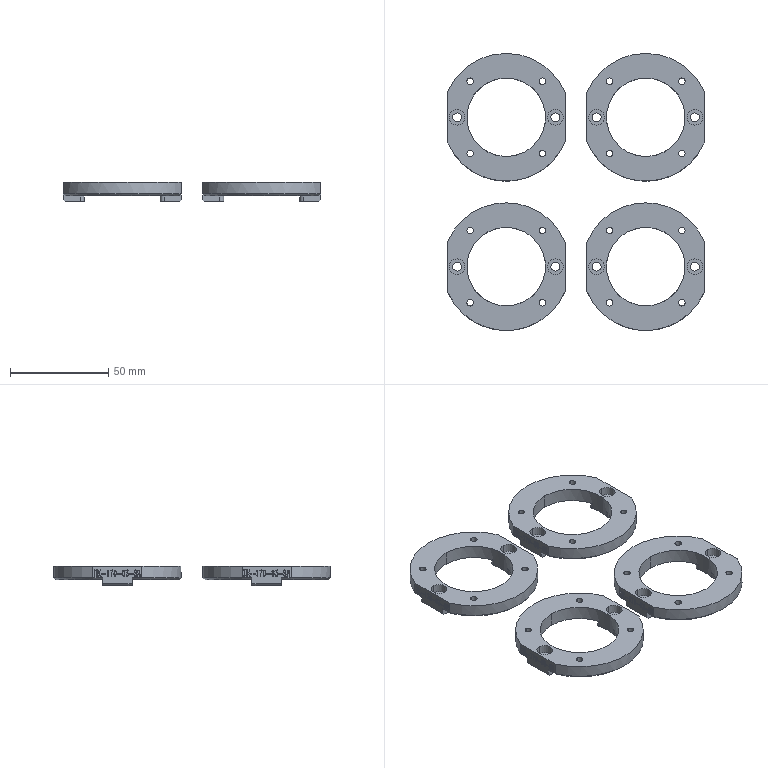NC program | NX | posted with a generic post | part box 131 x 141 x 10 mm
Lines 1 to 797 of 14293:
N10 G17 G21 G94 G90
(ZLEVEL_PROFILE_COPY_1_COPY , TOOL : D10)
N12 T15 M6
N14 G54
N16 G17 G0 G90 X-41.889 Y-75.045 S9500 M3
N18 G43 Z30. H15
N20 Z1.5
N22 G94 G1 X-42.763 Y-74.922 Z1.454 F1000.
N24 X-46.803 Y-73.892 Z1.235
N26 X-50.704 Y-72.422 Z1.017
N28 X-54.419 Y-70.528 Z0.798
N30 X-57.902 Y-68.235 Z0.58
N32 X-61.109 Y-65.572 Z0.361
N34 X-64.002 Y-62.569 Z0.143
N36 X-66.545 Y-59.265 Z-0.076
N38 X-68.143 Y-56.72 Z-0.233
N40 X-69.63 Y-53.848 Z-0.403
N42 X-70.208 Y-52.462 Z-0.482
N44 X-70.421 Y-51.95 Z-0.511
N46 X-70.6 Y-51.054 Z-0.558
N48 Y-50.5 Z-0.588
N50 Y-25.5 F3000.
N52 G2 X-70.208 Y-23.538 R5.1
N54 X-0.792 Y-23.538 R37.6
N56 X-0.4 Y-25.5 R5.1
N58 G1 Y-50.5
N60 G2 X-0.792 Y-52.462 R5.1
N62 X-70.208 Y-52.462 R37.6
N64 X-70.6 Y-50.5 R5.1
N66 G1 Y-25.5 Z-0.65
N68 X-70.575 Y-24.997 Z-0.651
N70 X-70.501 Y-24.5 Z-0.653
N72 X-70.378 Y-24.012 Z-0.654
N74 X-70.208 Y-23.538 Z-0.655
N76 X-69.614 Y-22.19 Z-0.659
N78 X-68.969 Y-20.865 Z-0.662
N80 X-68.272 Y-19.567 Z-0.666
N82 X-67.524 Y-18.297 Z-0.67
N84 X-66.727 Y-17.057 Z-0.673
N86 X-65.883 Y-15.85 Z-0.677
N88 X-64.992 Y-14.676 Z-0.681
N90 X-64.055 Y-13.538 Z-0.685
N92 X-63.075 Y-12.438 Z-0.688
N94 X-62.052 Y-11.377 Z-0.692
N96 X-60.988 Y-10.358 Z-0.696
N98 X-59.886 Y-9.38 Z-0.699
N100 X-58.745 Y-8.447 Z-0.703
N102 X-57.57 Y-7.558 Z-0.707
N104 X-56.36 Y-6.717 Z-0.71
N106 X-55.118 Y-5.924 Z-0.714
N108 X-53.846 Y-5.18 Z-0.718
N110 X-52.546 Y-4.486 Z-0.721
N112 X-51.22 Y-3.844 Z-0.725
N114 X-49.869 Y-3.254 Z-0.729
N116 X-48.497 Y-2.718 Z-0.732
N118 X-47.104 Y-2.235 Z-0.736
N120 X-45.694 Y-1.808 Z-0.74
N122 X-44.268 Y-1.437 Z-0.744
N124 X-42.829 Y-1.121 Z-0.747
N126 X-41.378 Y-0.862 Z-0.751
N128 X-39.918 Y-0.66 Z-0.755
N130 X-38.452 Y-0.516 Z-0.758
N132 X-36.981 Y-0.429 Z-0.762
N134 X-35.508 Y-0.4 Z-0.766
N136 X-34.034 Y-0.429 Z-0.769
N138 X-32.562 Y-0.515 Z-0.773
N140 X-31.095 Y-0.659 Z-0.777
N142 X-29.635 Y-0.86 Z-0.78
N144 X-28.184 Y-1.119 Z-0.784
N146 X-26.744 Y-1.434 Z-0.788
N148 X-25.317 Y-1.805 Z-0.791
N150 X-23.906 Y-2.232 Z-0.795
N152 X-22.513 Y-2.714 Z-0.799
N154 X-21.14 Y-3.25 Z-0.802
N156 X-19.789 Y-3.84 Z-0.806
N158 X-18.462 Y-4.482 Z-0.81
N160 X-17.161 Y-5.175 Z-0.814
N162 X-15.889 Y-5.919 Z-0.817
N164 X-14.646 Y-6.713 Z-0.821
N166 X-13.436 Y-7.554 Z-0.825
N168 X-12.26 Y-8.442 Z-0.828
N170 X-11.119 Y-9.376 Z-0.832
N172 X-10.016 Y-10.354 Z-0.836
N174 X-8.952 Y-11.374 Z-0.839
N176 X-7.928 Y-12.435 Z-0.843
N178 X-6.948 Y-13.535 Z-0.847
N180 X-6.011 Y-14.673 Z-0.85
N182 X-5.119 Y-15.847 Z-0.854
N184 X-4.274 Y-17.055 Z-0.858
N186 X-3.477 Y-18.295 Z-0.861
N188 X-2.729 Y-19.565 Z-0.865
N190 X-2.032 Y-20.864 Z-0.869
N192 X-1.386 Y-22.189 Z-0.873
N194 X-0.792 Y-23.538 Z-0.876
N196 X-0.622 Y-24.012 Z-0.877
N198 X-0.499 Y-24.5 Z-0.879
N200 X-0.425 Y-24.997 Z-0.88
N202 X-0.4 Y-25.5 Z-0.881
N204 Y-50.5 Z-0.944
N206 X-0.425 Y-51.003 Z-0.945
N208 X-0.499 Y-51.5 Z-0.946
N210 X-0.622 Y-51.988 Z-0.948
N212 X-0.792 Y-52.462 Z-0.949
N214 X-1.383 Y-53.805 Z-0.952
N216 X-2.026 Y-55.125 Z-0.956
N218 X-2.72 Y-56.418 Z-0.96
N220 X-3.464 Y-57.683 Z-0.963
N222 X-4.256 Y-58.919 Z-0.967
N224 X-5.097 Y-60.122 Z-0.971
N226 X-5.983 Y-61.292 Z-0.975
N228 X-6.915 Y-62.426 Z-0.978
N230 X-7.89 Y-63.523 Z-0.982
N232 X-8.907 Y-64.581 Z-0.986
N234 X-9.965 Y-65.599 Z-0.989
N236 X-11.061 Y-66.575 Z-0.993
N238 X-12.195 Y-67.507 Z-0.997
N240 X-13.364 Y-68.394 Z-1.
N242 X-14.568 Y-69.234 Z-1.004
N244 X-15.803 Y-70.028 Z-1.008
N246 X-17.068 Y-70.772 Z-1.011
N248 X-18.361 Y-71.466 Z-1.015
N250 X-19.68 Y-72.11 Z-1.019
N252 X-21.023 Y-72.701 Z-1.022
N254 X-22.389 Y-73.24 Z-1.026
N256 X-23.774 Y-73.725 Z-1.03
N258 X-25.177 Y-74.155 Z-1.033
N260 X-26.596 Y-74.531 Z-1.037
N262 X-28.029 Y-74.85 Z-1.041
N264 X-29.473 Y-75.114 Z-1.044
N266 X-30.926 Y-75.321 Z-1.048
N268 X-32.386 Y-75.471 Z-1.052
N270 X-33.851 Y-75.564 Z-1.055
N272 X-35.318 Y-75.6 Z-1.059
N274 X-36.786 Y-75.578 Z-1.063
N276 X-38.251 Y-75.499 Z-1.066
N278 X-39.713 Y-75.363 Z-1.07
N280 X-41.168 Y-75.17 Z-1.074
N282 X-42.614 Y-74.921 Z-1.077
N284 X-44.05 Y-74.615 Z-1.081
N286 X-45.472 Y-74.254 Z-1.085
N288 X-46.879 Y-73.837 Z-1.088
N290 X-48.269 Y-73.365 Z-1.092
N292 X-49.64 Y-72.84 Z-1.096
N294 X-50.989 Y-72.262 Z-1.099
N296 X-52.314 Y-71.631 Z-1.103
N298 X-53.614 Y-70.949 Z-1.107
N300 X-54.886 Y-70.217 Z-1.11
N302 X-56.129 Y-69.436 Z-1.114
N304 X-57.34 Y-68.607 Z-1.118
N306 X-58.518 Y-67.731 Z-1.121
N308 X-59.661 Y-66.81 Z-1.125
N310 X-60.767 Y-65.845 Z-1.129
N312 X-61.834 Y-64.838 Z-1.132
N314 X-62.862 Y-63.789 Z-1.136
N316 X-63.847 Y-62.702 Z-1.14
N318 X-64.79 Y-61.577 Z-1.143
N320 X-65.688 Y-60.416 Z-1.147
N322 X-66.54 Y-59.22 Z-1.151
N324 X-67.344 Y-57.993 Z-1.154
N326 X-67.885 Y-57.105 Z-1.157
N328 X-68.4 Y-56.203 Z-1.16
N330 X-68.891 Y-55.287 Z-1.162
N332 X-69.356 Y-54.357 Z-1.165
N334 X-69.795 Y-53.415 Z-1.167
N336 X-70.208 Y-52.462 Z-1.17
N338 X-70.378 Y-51.988 Z-1.171
N340 X-70.501 Y-51.5 Z-1.172
N342 X-70.575 Y-51.003 Z-1.174
N344 X-70.6 Y-50.5 Z-1.175
N346 Y-25.5 Z-1.238
N348 X-70.575 Y-24.997 Z-1.239
N350 X-70.501 Y-24.5 Z-1.24
N352 X-70.378 Y-24.012 Z-1.241
N354 X-70.208 Y-23.538 Z-1.243
N356 X-69.614 Y-22.19 Z-1.246
N358 X-68.969 Y-20.865 Z-1.25
N360 X-68.272 Y-19.567 Z-1.254
N362 X-67.524 Y-18.297 Z-1.257
N364 X-66.727 Y-17.057 Z-1.261
N366 X-65.883 Y-15.85 Z-1.265
N368 X-64.992 Y-14.676 Z-1.268
N370 X-64.055 Y-13.538 Z-1.272
N372 X-63.075 Y-12.438 Z-1.276
N374 X-62.052 Y-11.377 Z-1.279
N376 X-60.988 Y-10.358 Z-1.283
N378 X-59.886 Y-9.38 Z-1.287
N380 X-58.745 Y-8.447 Z-1.29
N382 X-57.57 Y-7.558 Z-1.294
N384 X-56.36 Y-6.717 Z-1.298
N386 X-55.118 Y-5.924 Z-1.302
N388 X-53.846 Y-5.18 Z-1.305
N390 X-52.546 Y-4.486 Z-1.309
N392 X-51.22 Y-3.844 Z-1.313
N394 X-49.869 Y-3.254 Z-1.316
N396 X-48.497 Y-2.718 Z-1.32
N398 X-47.104 Y-2.235 Z-1.324
N400 X-45.694 Y-1.808 Z-1.327
N402 X-44.268 Y-1.437 Z-1.331
N404 X-42.829 Y-1.121 Z-1.335
N406 X-41.378 Y-0.862 Z-1.338
N408 X-39.918 Y-0.66 Z-1.342
N410 X-38.452 Y-0.516 Z-1.346
N412 X-36.981 Y-0.429 Z-1.349
N414 X-35.508 Y-0.4 Z-1.353
N416 X-34.034 Y-0.429 Z-1.357
N418 X-32.562 Y-0.515 Z-1.36
N420 X-31.095 Y-0.659 Z-1.364
N422 X-29.635 Y-0.86 Z-1.368
N424 X-28.184 Y-1.119 Z-1.372
N426 X-26.744 Y-1.434 Z-1.375
N428 X-25.317 Y-1.805 Z-1.379
N430 X-23.906 Y-2.232 Z-1.383
N432 X-22.513 Y-2.714 Z-1.386
N434 X-21.14 Y-3.25 Z-1.39
N436 X-19.789 Y-3.84 Z-1.394
N438 X-18.462 Y-4.482 Z-1.397
N440 X-17.161 Y-5.175 Z-1.401
N442 X-15.889 Y-5.919 Z-1.405
N444 X-14.646 Y-6.713 Z-1.408
N446 X-13.436 Y-7.554 Z-1.412
N448 X-12.26 Y-8.442 Z-1.416
N450 X-11.119 Y-9.376 Z-1.419
N452 X-10.016 Y-10.354 Z-1.423
N454 X-8.952 Y-11.374 Z-1.427
N456 X-7.928 Y-12.435 Z-1.431
N458 X-6.948 Y-13.535 Z-1.434
N460 X-6.011 Y-14.673 Z-1.438
N462 X-5.119 Y-15.847 Z-1.442
N464 X-4.274 Y-17.055 Z-1.445
N466 X-3.477 Y-18.295 Z-1.449
N468 X-2.729 Y-19.565 Z-1.453
N470 X-2.032 Y-20.864 Z-1.456
N472 X-1.386 Y-22.189 Z-1.46
N474 X-0.792 Y-23.538 Z-1.464
N476 X-0.622 Y-24.012 Z-1.465
N478 X-0.499 Y-24.5 Z-1.466
N480 X-0.425 Y-24.997 Z-1.467
N482 X-0.4 Y-25.5 Z-1.469
N484 Y-50.5 Z-1.531
N486 X-0.425 Y-51.003 Z-1.533
N488 X-0.499 Y-51.5 Z-1.534
N490 X-0.622 Y-51.988 Z-1.535
N492 X-0.792 Y-52.462 Z-1.536
N494 X-1.383 Y-53.805 Z-1.54
N496 X-2.026 Y-55.125 Z-1.544
N498 X-2.72 Y-56.418 Z-1.547
N500 X-3.464 Y-57.683 Z-1.551
N502 X-4.256 Y-58.919 Z-1.555
N504 X-5.097 Y-60.122 Z-1.558
N506 X-5.983 Y-61.292 Z-1.562
N508 X-6.915 Y-62.426 Z-1.566
N510 X-7.89 Y-63.523 Z-1.569
N512 X-8.907 Y-64.581 Z-1.573
N514 X-9.965 Y-65.599 Z-1.577
N516 X-11.061 Y-66.575 Z-1.58
N518 X-12.195 Y-67.507 Z-1.584
N520 X-13.364 Y-68.394 Z-1.588
N522 X-14.568 Y-69.234 Z-1.591
N524 X-15.803 Y-70.028 Z-1.595
N526 X-17.068 Y-70.772 Z-1.599
N528 X-18.361 Y-71.466 Z-1.602
N530 X-19.68 Y-72.11 Z-1.606
N532 X-21.023 Y-72.701 Z-1.61
N534 X-22.389 Y-73.24 Z-1.613
N536 X-23.774 Y-73.725 Z-1.617
N538 X-25.177 Y-74.155 Z-1.621
N540 X-26.596 Y-74.531 Z-1.624
N542 X-28.029 Y-74.85 Z-1.628
N544 X-29.473 Y-75.114 Z-1.632
N546 X-30.926 Y-75.321 Z-1.635
N548 X-32.386 Y-75.471 Z-1.639
N550 X-33.851 Y-75.564 Z-1.643
N552 X-35.318 Y-75.6 Z-1.646
N554 X-36.786 Y-75.578 Z-1.65
N556 X-38.251 Y-75.499 Z-1.654
N558 X-39.713 Y-75.363 Z-1.657
N560 X-41.168 Y-75.17 Z-1.661
N562 X-42.614 Y-74.921 Z-1.665
N564 X-44.05 Y-74.615 Z-1.668
N566 X-45.472 Y-74.254 Z-1.672
N568 X-46.879 Y-73.837 Z-1.676
N570 X-48.269 Y-73.365 Z-1.679
N572 X-49.64 Y-72.84 Z-1.683
N574 X-50.989 Y-72.262 Z-1.687
N576 X-52.314 Y-71.631 Z-1.69
N578 X-53.614 Y-70.949 Z-1.694
N580 X-54.886 Y-70.217 Z-1.698
N582 X-56.129 Y-69.436 Z-1.701
N584 X-57.34 Y-68.607 Z-1.705
N586 X-58.518 Y-67.731 Z-1.709
N588 X-59.661 Y-66.81 Z-1.713
N590 X-60.767 Y-65.845 Z-1.716
N592 X-61.834 Y-64.838 Z-1.72
N594 X-62.862 Y-63.789 Z-1.724
N596 X-63.847 Y-62.702 Z-1.727
N598 X-64.79 Y-61.577 Z-1.731
N600 X-65.688 Y-60.416 Z-1.735
N602 X-66.54 Y-59.22 Z-1.738
N604 X-67.344 Y-57.993 Z-1.742
N606 X-67.885 Y-57.105 Z-1.744
N608 X-68.4 Y-56.203 Z-1.747
N610 X-68.891 Y-55.287 Z-1.75
N612 X-69.356 Y-54.357 Z-1.752
N614 X-69.795 Y-53.415 Z-1.755
N616 X-70.208 Y-52.462 Z-1.757
N618 X-70.378 Y-51.988 Z-1.759
N620 X-70.501 Y-51.5 Z-1.76
N622 X-70.575 Y-51.003 Z-1.761
N624 X-70.6 Y-50.5 Z-1.763
N626 Y-25.5 Z-1.825
N628 X-70.575 Y-24.997 Z-1.826
N630 X-70.501 Y-24.5 Z-1.828
N632 X-70.378 Y-24.012 Z-1.829
N634 X-70.208 Y-23.538 Z-1.83
N636 X-69.614 Y-22.19 Z-1.834
N638 X-68.969 Y-20.865 Z-1.837
N640 X-68.272 Y-19.567 Z-1.841
N642 X-67.524 Y-18.297 Z-1.845
N644 X-66.727 Y-17.057 Z-1.848
N646 X-65.883 Y-15.85 Z-1.852
N648 X-64.992 Y-14.676 Z-1.856
N650 X-64.055 Y-13.538 Z-1.86
N652 X-63.075 Y-12.438 Z-1.863
N654 X-62.052 Y-11.377 Z-1.867
N656 X-60.988 Y-10.358 Z-1.871
N658 X-59.886 Y-9.38 Z-1.874
N660 X-58.745 Y-8.447 Z-1.878
N662 X-57.57 Y-7.558 Z-1.882
N664 X-56.36 Y-6.717 Z-1.885
N666 X-55.118 Y-5.924 Z-1.889
N668 X-53.846 Y-5.18 Z-1.893
N670 X-52.546 Y-4.486 Z-1.896
N672 X-51.22 Y-3.844 Z-1.9
N674 X-49.869 Y-3.254 Z-1.904
N676 X-48.497 Y-2.718 Z-1.907
N678 X-47.104 Y-2.235 Z-1.911
N680 X-45.694 Y-1.808 Z-1.915
N682 X-44.268 Y-1.437 Z-1.919
N684 X-42.829 Y-1.121 Z-1.922
N686 X-41.378 Y-0.862 Z-1.926
N688 X-39.918 Y-0.66 Z-1.93
N690 X-38.452 Y-0.516 Z-1.933
N692 X-36.981 Y-0.429 Z-1.937
N694 X-35.508 Y-0.4 Z-1.941
N696 X-34.034 Y-0.429 Z-1.944
N698 X-32.562 Y-0.515 Z-1.948
N700 X-31.095 Y-0.659 Z-1.952
N702 X-29.635 Y-0.86 Z-1.955
N704 X-28.184 Y-1.119 Z-1.959
N706 X-26.744 Y-1.434 Z-1.963
N708 X-25.317 Y-1.805 Z-1.966
N710 X-23.906 Y-2.232 Z-1.97
N712 X-22.513 Y-2.714 Z-1.974
N714 X-21.14 Y-3.25 Z-1.977
N716 X-19.789 Y-3.84 Z-1.981
N718 X-18.462 Y-4.482 Z-1.985
N720 X-17.161 Y-5.175 Z-1.989
N722 X-15.889 Y-5.919 Z-1.992
N724 X-14.646 Y-6.713 Z-1.996
N726 X-13.436 Y-7.554 Z-2.
N728 X-12.26 Y-8.442 Z-2.003
N730 X-11.119 Y-9.376 Z-2.007
N732 X-10.016 Y-10.354 Z-2.011
N734 X-8.952 Y-11.374 Z-2.014
N736 X-7.928 Y-12.435 Z-2.018
N738 X-6.948 Y-13.535 Z-2.022
N740 X-6.011 Y-14.673 Z-2.025
N742 X-5.119 Y-15.847 Z-2.029
N744 X-4.274 Y-17.055 Z-2.033
N746 X-3.477 Y-18.295 Z-2.036
N748 X-2.729 Y-19.565 Z-2.04
N750 X-2.032 Y-20.864 Z-2.044
N752 X-1.386 Y-22.189 Z-2.048
N754 X-0.792 Y-23.538 Z-2.051
N756 X-0.622 Y-24.012 Z-2.052
N758 X-0.499 Y-24.5 Z-2.054
N760 X-0.425 Y-24.997 Z-2.055
N762 X-0.4 Y-25.5 Z-2.056
N764 Y-50.5 Z-2.119
N766 X-0.425 Y-51.003 Z-2.12
N768 X-0.499 Y-51.5 Z-2.121
N770 X-0.622 Y-51.988 Z-2.123
N772 X-0.792 Y-52.462 Z-2.124
N774 X-1.383 Y-53.805 Z-2.127
N776 X-2.026 Y-55.125 Z-2.131
N778 X-2.72 Y-56.418 Z-2.135
N780 X-3.464 Y-57.683 Z-2.138
N782 X-4.256 Y-58.919 Z-2.142
N784 X-5.097 Y-60.122 Z-2.146
N786 X-5.983 Y-61.292 Z-2.15
N788 X-6.915 Y-62.426 Z-2.153
N790 X-7.89 Y-63.523 Z-2.157
N792 X-8.907 Y-64.581 Z-2.161
N794 X-9.965 Y-65.599 Z-2.164
N796 X-11.061 Y-66.575 Z-2.168
N798 X-12.195 Y-67.507 Z-2.172
N800 X-13.364 Y-68.394 Z-2.175
N802 X-14.568 Y-69.234 Z-2.179
N804 X-15.803 Y-70.028 Z-2.183
N806 X-17.068 Y-70.772 Z-2.186
N808 X-18.361 Y-71.466 Z-2.19
N810 X-19.68 Y-72.11 Z-2.194
N812 X-21.023 Y-72.701 Z-2.197
N814 X-22.389 Y-73.24 Z-2.201
N816 X-23.774 Y-73.725 Z-2.205
N818 X-25.177 Y-74.155 Z-2.208
N820 X-26.596 Y-74.531 Z-2.212
N822 X-28.029 Y-74.85 Z-2.216
N824 X-29.473 Y-75.114 Z-2.219
N826 X-30.926 Y-75.321 Z-2.223
N828 X-32.386 Y-75.471 Z-2.227
N830 X-33.851 Y-75.564 Z-2.23
N832 X-35.318 Y-75.6 Z-2.234
N834 X-36.786 Y-75.578 Z-2.238
N836 X-38.251 Y-75.499 Z-2.241
N838 X-39.713 Y-75.363 Z-2.245
N840 X-41.168 Y-75.17 Z-2.249
N842 X-42.614 Y-74.921 Z-2.252
N844 X-44.05 Y-74.615 Z-2.256
N846 X-45.472 Y-74.254 Z-2.26
N848 X-46.879 Y-73.837 Z-2.263
N850 X-48.269 Y-73.365 Z-2.267
N852 X-49.64 Y-72.84 Z-2.271
N854 X-50.989 Y-72.262 Z-2.274
N856 X-52.314 Y-71.631 Z-2.278
N858 X-53.614 Y-70.949 Z-2.282
N860 X-54.886 Y-70.217 Z-2.285
N862 X-56.129 Y-69.436 Z-2.289
N864 X-57.34 Y-68.607 Z-2.293
N866 X-58.518 Y-67.731 Z-2.296
N868 X-59.661 Y-66.81 Z-2.3
N870 X-60.767 Y-65.845 Z-2.304
N872 X-61.834 Y-64.838 Z-2.307
N874 X-62.862 Y-63.789 Z-2.311
N876 X-63.847 Y-62.702 Z-2.315
N878 X-64.79 Y-61.577 Z-2.318
N880 X-65.688 Y-60.416 Z-2.322
N882 X-66.54 Y-59.22 Z-2.326
N884 X-67.344 Y-57.993 Z-2.329
N886 X-67.885 Y-57.105 Z-2.332
N888 X-68.4 Y-56.203 Z-2.335
N890 X-68.891 Y-55.287 Z-2.337
N892 X-69.356 Y-54.357 Z-2.34
N894 X-69.795 Y-53.415 Z-2.342
N896 X-70.208 Y-52.462 Z-2.345
N898 X-70.378 Y-51.988 Z-2.346
N900 X-70.501 Y-51.5 Z-2.347
N902 X-70.575 Y-51.003 Z-2.349
N904 X-70.6 Y-50.5 Z-2.35
N906 Y-25.5 Z-2.413
N908 X-70.575 Y-24.997 Z-2.414
N910 X-70.501 Y-24.5 Z-2.415
N912 X-70.378 Y-24.012 Z-2.416
N914 X-70.208 Y-23.538 Z-2.418
N916 X-69.614 Y-22.19 Z-2.421
N918 X-68.969 Y-20.865 Z-2.425
N920 X-68.272 Y-19.567 Z-2.429
N922 X-67.524 Y-18.297 Z-2.432
N924 X-66.727 Y-17.057 Z-2.436
N926 X-65.883 Y-15.85 Z-2.44
N928 X-64.992 Y-14.676 Z-2.443
N930 X-64.055 Y-13.538 Z-2.447
N932 X-63.075 Y-12.438 Z-2.451
N934 X-62.052 Y-11.377 Z-2.454
N936 X-60.988 Y-10.358 Z-2.458
N938 X-59.886 Y-9.38 Z-2.462
N940 X-58.745 Y-8.447 Z-2.465
N942 X-57.57 Y-7.558 Z-2.469
N944 X-56.36 Y-6.717 Z-2.473
N946 X-55.118 Y-5.924 Z-2.477
N948 X-53.846 Y-5.18 Z-2.48
N950 X-52.546 Y-4.486 Z-2.484
N952 X-51.22 Y-3.844 Z-2.488
N954 X-49.869 Y-3.254 Z-2.491
N956 X-48.497 Y-2.718 Z-2.495
N958 X-47.104 Y-2.235 Z-2.499
N960 X-45.694 Y-1.808 Z-2.502
N962 X-44.268 Y-1.437 Z-2.506
N964 X-42.829 Y-1.121 Z-2.51
N966 X-41.378 Y-0.862 Z-2.513
N968 X-39.918 Y-0.66 Z-2.517
N970 X-38.452 Y-0.516 Z-2.521
N972 X-36.981 Y-0.429 Z-2.524
N974 X-35.508 Y-0.4 Z-2.528
N976 X-34.034 Y-0.429 Z-2.532
N978 X-32.562 Y-0.515 Z-2.535
N980 X-31.095 Y-0.659 Z-2.539
N982 X-29.635 Y-0.86 Z-2.543
N984 X-28.184 Y-1.119 Z-2.547
N986 X-26.744 Y-1.434 Z-2.55
N988 X-25.317 Y-1.805 Z-2.554
N990 X-23.906 Y-2.232 Z-2.558
N992 X-22.513 Y-2.714 Z-2.561
N994 X-21.14 Y-3.25 Z-2.565
N996 X-19.789 Y-3.84 Z-2.569
N998 X-18.462 Y-4.482 Z-2.572
N1000 X-17.161 Y-5.175 Z-2.576
N1002 X-15.889 Y-5.919 Z-2.58
N1004 X-14.646 Y-6.713 Z-2.583
N1006 X-13.436 Y-7.554 Z-2.587
N1008 X-12.26 Y-8.442 Z-2.591
N1010 X-11.119 Y-9.376 Z-2.594
N1012 X-10.016 Y-10.354 Z-2.598
N1014 X-8.952 Y-11.374 Z-2.602
N1016 X-7.928 Y-12.435 Z-2.606
N1018 X-6.948 Y-13.535 Z-2.609
N1020 X-6.011 Y-14.673 Z-2.613
N1022 X-5.119 Y-15.847 Z-2.617
N1024 X-4.274 Y-17.055 Z-2.62
N1026 X-3.477 Y-18.295 Z-2.624
N1028 X-2.729 Y-19.565 Z-2.628
N1030 X-2.032 Y-20.864 Z-2.631
N1032 X-1.386 Y-22.189 Z-2.635
N1034 X-0.792 Y-23.538 Z-2.639
N1036 X-0.622 Y-24.012 Z-2.64
N1038 X-0.499 Y-24.5 Z-2.641
N1040 X-0.425 Y-24.997 Z-2.642
N1042 X-0.4 Y-25.5 Z-2.644
N1044 Y-50.5 Z-2.706
N1046 X-0.425 Y-51.003 Z-2.708
N1048 X-0.499 Y-51.5 Z-2.709
N1050 X-0.622 Y-51.988 Z-2.71
N1052 X-0.792 Y-52.462 Z-2.711
N1054 X-1.383 Y-53.805 Z-2.715
N1056 X-2.026 Y-55.125 Z-2.719
N1058 X-2.72 Y-56.418 Z-2.722
N1060 X-3.464 Y-57.683 Z-2.726
N1062 X-4.256 Y-58.919 Z-2.73
N1064 X-5.097 Y-60.122 Z-2.733
N1066 X-5.983 Y-61.292 Z-2.737
N1068 X-6.915 Y-62.426 Z-2.741
N1070 X-7.89 Y-63.523 Z-2.744
N1072 X-8.907 Y-64.581 Z-2.748
N1074 X-9.965 Y-65.599 Z-2.752
N1076 X-11.061 Y-66.575 Z-2.755
N1078 X-12.195 Y-67.507 Z-2.759
N1080 X-13.364 Y-68.394 Z-2.763
N1082 X-14.568 Y-69.234 Z-2.766
N1084 X-15.803 Y-70.028 Z-2.77
N1086 X-17.068 Y-70.772 Z-2.774
N1088 X-18.361 Y-71.466 Z-2.777
N1090 X-19.68 Y-72.11 Z-2.781
N1092 X-21.023 Y-72.701 Z-2.785
N1094 X-22.389 Y-73.24 Z-2.788
N1096 X-23.774 Y-73.725 Z-2.792
N1098 X-25.177 Y-74.155 Z-2.796
N1100 X-26.596 Y-74.531 Z-2.799
N1102 X-28.029 Y-74.85 Z-2.803
N1104 X-29.473 Y-75.114 Z-2.807
N1106 X-30.926 Y-75.321 Z-2.81
N1108 X-32.386 Y-75.471 Z-2.814
N1110 X-33.851 Y-75.564 Z-2.818
N1112 X-35.318 Y-75.6 Z-2.821
N1114 X-36.786 Y-75.578 Z-2.825
N1116 X-38.251 Y-75.499 Z-2.829
N1118 X-39.713 Y-75.363 Z-2.832
N1120 X-41.168 Y-75.17 Z-2.836
N1122 X-42.614 Y-74.921 Z-2.84
N1124 X-44.05 Y-74.615 Z-2.843
N1126 X-45.472 Y-74.254 Z-2.847
N1128 X-46.879 Y-73.837 Z-2.851
N1130 X-48.269 Y-73.365 Z-2.854
N1132 X-49.64 Y-72.84 Z-2.858
N1134 X-50.989 Y-72.262 Z-2.862
N1136 X-52.314 Y-71.631 Z-2.865
N1138 X-53.614 Y-70.949 Z-2.869
N1140 X-54.886 Y-70.217 Z-2.873
N1142 X-56.129 Y-69.436 Z-2.876
N1144 X-57.34 Y-68.607 Z-2.88
N1146 X-58.518 Y-67.731 Z-2.884
N1148 X-59.661 Y-66.81 Z-2.888
N1150 X-60.767 Y-65.845 Z-2.891
N1152 X-61.834 Y-64.838 Z-2.895
N1154 X-62.862 Y-63.789 Z-2.899
N1156 X-63.847 Y-62.702 Z-2.902
N1158 X-64.79 Y-61.577 Z-2.906
N1160 X-65.688 Y-60.416 Z-2.91
N1162 X-66.54 Y-59.22 Z-2.913
N1164 X-67.344 Y-57.993 Z-2.917
N1166 X-67.885 Y-57.105 Z-2.919
N1168 X-68.4 Y-56.203 Z-2.922
N1170 X-68.891 Y-55.287 Z-2.925
N1172 X-69.356 Y-54.357 Z-2.927
N1174 X-69.795 Y-53.415 Z-2.93
N1176 X-70.208 Y-52.462 Z-2.932
N1178 X-70.378 Y-51.988 Z-2.934
N1180 X-70.501 Y-51.5 Z-2.935
N1182 X-70.575 Y-51.003 Z-2.936
N1184 X-70.6 Y-50.5 Z-2.938
N1186 Y-25.5 Z-3.
N1188 X-70.575 Y-24.997 Z-3.001
N1190 X-70.501 Y-24.5 Z-3.003
N1192 X-70.378 Y-24.012 Z-3.004
N1194 X-70.208 Y-23.538 Z-3.005
N1196 X-69.614 Y-22.19 Z-3.009
N1198 X-68.969 Y-20.865 Z-3.012
N1200 X-68.272 Y-19.567 Z-3.016
N1202 X-67.524 Y-18.297 Z-3.02
N1204 X-66.727 Y-17.057 Z-3.023
N1206 X-65.883 Y-15.85 Z-3.027
N1208 X-64.992 Y-14.676 Z-3.031
N1210 X-64.055 Y-13.538 Z-3.035
N1212 X-63.075 Y-12.438 Z-3.038
N1214 X-62.052 Y-11.377 Z-3.042
N1216 X-60.988 Y-10.358 Z-3.046
N1218 X-59.886 Y-9.38 Z-3.049
N1220 X-58.745 Y-8.447 Z-3.053
N1222 X-57.57 Y-7.558 Z-3.057
N1224 X-56.36 Y-6.717 Z-3.06
N1226 X-55.118 Y-5.924 Z-3.064
N1228 X-53.846 Y-5.18 Z-3.068
N1230 X-52.546 Y-4.486 Z-3.071
N1232 X-51.22 Y-3.844 Z-3.075
N1234 X-49.869 Y-3.254 Z-3.079
N1236 X-48.497 Y-2.718 Z-3.082
N1238 X-47.104 Y-2.235 Z-3.086
N1240 X-45.694 Y-1.808 Z-3.09
N1242 X-44.268 Y-1.437 Z-3.094
N1244 X-42.829 Y-1.121 Z-3.097
N1246 X-41.378 Y-0.862 Z-3.101
N1248 X-39.918 Y-0.66 Z-3.105
N1250 X-38.452 Y-0.516 Z-3.108
N1252 X-36.981 Y-0.429 Z-3.112
N1254 X-35.508 Y-0.4 Z-3.116
N1256 X-34.034 Y-0.429 Z-3.119
N1258 X-32.562 Y-0.515 Z-3.123
N1260 X-31.095 Y-0.659 Z-3.127
N1262 X-29.635 Y-0.86 Z-3.13
N1264 X-28.184 Y-1.119 Z-3.134
N1266 X-26.744 Y-1.434 Z-3.138
N1268 X-25.317 Y-1.805 Z-3.141
N1270 X-23.906 Y-2.232 Z-3.145
N1272 X-22.513 Y-2.714 Z-3.149
N1274 X-21.14 Y-3.25 Z-3.152
N1276 X-19.789 Y-3.84 Z-3.156
N1278 X-18.462 Y-4.482 Z-3.16
N1280 X-17.161 Y-5.175 Z-3.164
N1282 X-15.889 Y-5.919 Z-3.167
N1284 X-14.646 Y-6.713 Z-3.171
N1286 X-13.436 Y-7.554 Z-3.175
N1288 X-12.26 Y-8.442 Z-3.178
N1290 X-11.119 Y-9.376 Z-3.182
N1292 X-10.016 Y-10.354 Z-3.186
N1294 X-8.952 Y-11.374 Z-3.189
N1296 X-7.928 Y-12.435 Z-3.193
N1298 X-6.948 Y-13.535 Z-3.197
N1300 X-6.011 Y-14.673 Z-3.2
N1302 X-5.119 Y-15.847 Z-3.204
N1304 X-4.274 Y-17.055 Z-3.208
N1306 X-3.477 Y-18.295 Z-3.211
N1308 X-2.729 Y-19.565 Z-3.215
N1310 X-2.032 Y-20.864 Z-3.219
N1312 X-1.386 Y-22.189 Z-3.223
N1314 X-0.792 Y-23.538 Z-3.226
N1316 X-0.622 Y-24.012 Z-3.227
N1318 X-0.499 Y-24.5 Z-3.229
N1320 X-0.425 Y-24.997 Z-3.23
N1322 X-0.4 Y-25.5 Z-3.231
N1324 Y-50.5 Z-3.294
N1326 X-0.425 Y-51.003 Z-3.295
N1328 X-0.499 Y-51.5 Z-3.296
N1330 X-0.622 Y-51.988 Z-3.298
N1332 X-0.792 Y-52.462 Z-3.299
N1334 X-1.383 Y-53.805 Z-3.302
N1336 X-2.026 Y-55.125 Z-3.306
N1338 X-2.72 Y-56.418 Z-3.31
N1340 X-3.464 Y-57.683 Z-3.313
N1342 X-4.256 Y-58.919 Z-3.317
N1344 X-5.097 Y-60.122 Z-3.321
N1346 X-5.983 Y-61.292 Z-3.325
N1348 X-6.915 Y-62.426 Z-3.328
N1350 X-7.89 Y-63.523 Z-3.332
N1352 X-8.907 Y-64.581 Z-3.336
N1354 X-9.965 Y-65.599 Z-3.339
N1356 X-11.061 Y-66.575 Z-3.343
N1358 X-12.195 Y-67.507 Z-3.347
N1360 X-13.364 Y-68.394 Z-3.35
N1362 X-14.568 Y-69.234 Z-3.354
N1364 X-15.803 Y-70.028 Z-3.358
N1366 X-17.068 Y-70.772 Z-3.361
N1368 X-18.361 Y-71.466 Z-3.365
N1370 X-19.68 Y-72.11 Z-3.369
N1372 X-21.023 Y-72.701 Z-3.372
N1374 X-22.389 Y-73.24 Z-3.376
N1376 X-23.774 Y-73.725 Z-3.38
N1378 X-25.177 Y-74.155 Z-3.383
N1380 X-26.596 Y-74.531 Z-3.387
N1382 X-28.029 Y-74.85 Z-3.391
N1384 X-29.473 Y-75.114 Z-3.394
N1386 X-30.926 Y-75.321 Z-3.398
N1388 X-32.386 Y-75.471 Z-3.402
N1390 X-33.851 Y-75.564 Z-3.405
N1392 X-35.318 Y-75.6 Z-3.409
N1394 X-36.786 Y-75.578 Z-3.413
N1396 X-38.251 Y-75.499 Z-3.416
N1398 X-39.713 Y-75.363 Z-3.42
N1400 X-41.168 Y-75.17 Z-3.424
N1402 X-42.614 Y-74.921 Z-3.427
N1404 X-44.05 Y-74.615 Z-3.431
N1406 X-45.472 Y-74.254 Z-3.435
N1408 X-46.879 Y-73.837 Z-3.438
N1410 X-48.269 Y-73.365 Z-3.442
N1412 X-49.64 Y-72.84 Z-3.446
N1414 X-50.989 Y-72.262 Z-3.449
N1416 X-52.314 Y-71.631 Z-3.453
N1418 X-53.614 Y-70.949 Z-3.457
N1420 X-54.886 Y-70.217 Z-3.46
N1422 X-56.129 Y-69.436 Z-3.464
N1424 X-57.34 Y-68.607 Z-3.468
N1426 X-58.518 Y-67.731 Z-3.471
N1428 X-59.661 Y-66.81 Z-3.475
N1430 X-60.767 Y-65.845 Z-3.479
N1432 X-61.834 Y-64.838 Z-3.482
N1434 X-62.862 Y-63.789 Z-3.486
N1436 X-63.847 Y-62.702 Z-3.49
N1438 X-64.79 Y-61.577 Z-3.493
N1440 X-65.688 Y-60.416 Z-3.497
N1442 X-66.54 Y-59.22 Z-3.501
N1444 X-67.344 Y-57.993 Z-3.504
N1446 X-67.885 Y-57.105 Z-3.507
N1448 X-68.4 Y-56.203 Z-3.51
N1450 X-68.891 Y-55.287 Z-3.512
N1452 X-69.356 Y-54.357 Z-3.515
N1454 X-69.795 Y-53.415 Z-3.517
N1456 X-70.208 Y-52.462 Z-3.52
N1458 X-70.378 Y-51.988 Z-3.521
N1460 X-70.501 Y-51.5 Z-3.522
N1462 X-70.575 Y-51.003 Z-3.524
N1464 X-70.6 Y-50.5 Z-3.525
N1466 Y-25.5 Z-3.588
N1468 X-70.575 Y-24.997 Z-3.589
N1470 X-70.501 Y-24.5 Z-3.59
N1472 X-70.378 Y-24.012 Z-3.591
N1474 X-70.208 Y-23.538 Z-3.593
N1476 X-69.614 Y-22.19 Z-3.596
N1478 X-68.969 Y-20.865 Z-3.6
N1480 X-68.272 Y-19.567 Z-3.604
N1482 X-67.524 Y-18.297 Z-3.607
N1484 X-66.727 Y-17.057 Z-3.611
N1486 X-65.883 Y-15.85 Z-3.615
N1488 X-64.992 Y-14.676 Z-3.618
N1490 X-64.055 Y-13.538 Z-3.622
N1492 X-63.075 Y-12.438 Z-3.626
N1494 X-62.052 Y-11.377 Z-3.629
N1496 X-60.988 Y-10.358 Z-3.633
N1498 X-59.886 Y-9.38 Z-3.637
N1500 X-58.745 Y-8.447 Z-3.64
N1502 X-57.57 Y-7.558 Z-3.644
N1504 X-56.36 Y-6.717 Z-3.648
N1506 X-55.118 Y-5.924 Z-3.652
N1508 X-53.846 Y-5.18 Z-3.655
N1510 X-52.546 Y-4.486 Z-3.659
N1512 X-51.22 Y-3.844 Z-3.663
N1514 X-49.869 Y-3.254 Z-3.666
N1516 X-48.497 Y-2.718 Z-3.67
N1518 X-47.104 Y-2.235 Z-3.674
N1520 X-45.694 Y-1.808 Z-3.677
N1522 X-44.268 Y-1.437 Z-3.681
N1524 X-42.829 Y-1.121 Z-3.685
N1526 X-41.378 Y-0.862 Z-3.688
N1528 X-39.918 Y-0.66 Z-3.692
N1530 X-38.452 Y-0.516 Z-3.696
N1532 X-36.981 Y-0.429 Z-3.699
N1534 X-35.508 Y-0.4 Z-3.703
N1536 X-34.034 Y-0.429 Z-3.707
N1538 X-32.562 Y-0.515 Z-3.71
N1540 X-31.095 Y-0.659 Z-3.714
N1542 X-29.635 Y-0.86 Z-3.718
N1544 X-28.184 Y-1.119 Z-3.722
N1546 X-26.744 Y-1.434 Z-3.725
N1548 X-25.317 Y-1.805 Z-3.729
N1550 X-23.906 Y-2.232 Z-3.733
N1552 X-22.513 Y-2.714 Z-3.736
N1554 X-21.14 Y-3.25 Z-3.74
N1556 X-19.789 Y-3.84 Z-3.744
N1558 X-18.462 Y-4.482 Z-3.747
N1560 X-17.161 Y-5.175 Z-3.751
N1562 X-15.889 Y-5.919 Z-3.755
N1564 X-14.646 Y-6.713 Z-3.758
N1566 X-13.436 Y-7.554 Z-3.762
N1568 X-12.26 Y-8.442 Z-3.766
N1570 X-11.119 Y-9.376 Z-3.769
N1572 X-10.016 Y-10.354 Z-3.773
N1574 X-8.952 Y-11.374 Z-3.777
N1576 X-7.928 Y-12.435 Z-3.781
N1578 X-6.948 Y-13.535 Z-3.784
N1580 X-6.011 Y-14.673 Z-3.788
N1582 X-5.119 Y-15.847 Z-3.792
N1584 X-4.274 Y-17.055 Z-3.795
N1586 X-3.477 Y-18.295 Z-3.799
N1588 X-2.729 Y-19.565 Z-3.803
N1590 X-2.032 Y-20.864 Z-3.806
N1592 X-1.386 Y-22.189 Z-3.81